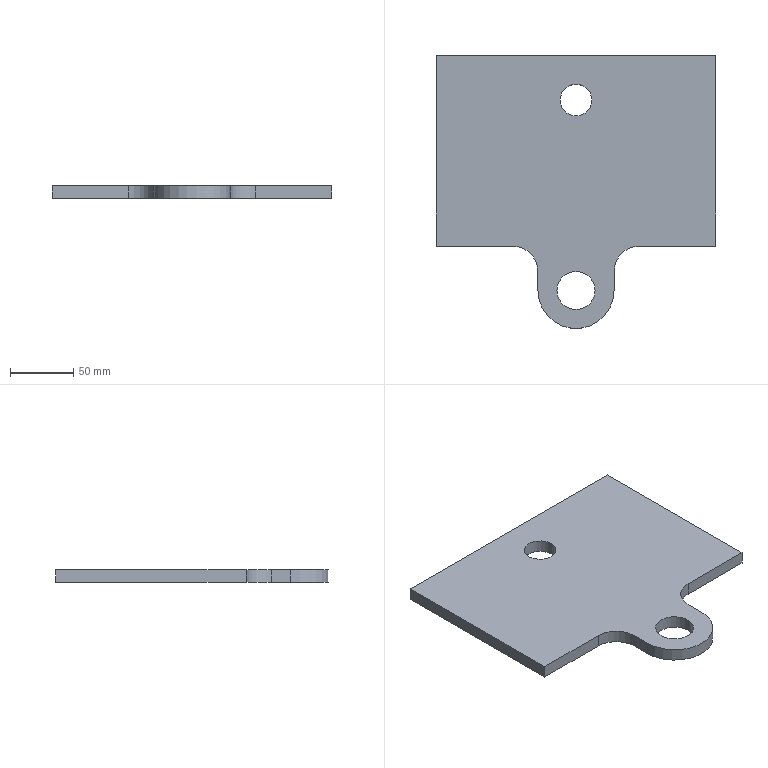Part | SolidWorks | features Extrusion 1, Fillet 1 | 1 solid | 16 faces | box 220 x 215 x 10 mm | volume 354877 mm3 | plane 9 | cylinder 7 | commonest cylinder face diameters 25 x2 30 x2 40 x2 60 x1
STEP:
#1=CARTESIAN_POINT('',(-12.5,40.,5.));
#2=VERTEX_POINT('',#1);
#3=CARTESIAN_POINT('',(12.5,40.,5.));
#4=VERTEX_POINT('',#3);
#5=CARTESIAN_POINT('',(0.,40.,5.));
#6=DIRECTION('',(0.,0.,1.));
#7=DIRECTION('',(1.,0.,0.));
#8=AXIS2_PLACEMENT_3D('',#5,#6,#7);
#9=CIRCLE('',#8,12.5);
#10=EDGE_CURVE('',#2,#4,#9,.T.);
#11=ORIENTED_EDGE('',*,*,#10,.T.);
#12=CARTESIAN_POINT('',(12.5,40.,-5.));
#13=VERTEX_POINT('',#12);
#14=CARTESIAN_POINT('',(12.5,40.,5.));
#15=DIRECTION('',(0.,0.,-1.));
#16=VECTOR('',#15,1000.);
#17=LINE('',#14,#16);
#18=EDGE_CURVE('',#4,#13,#17,.T.);
#19=ORIENTED_EDGE('',*,*,#18,.T.);
#20=CARTESIAN_POINT('',(-12.5,40.,-5.));
#21=VERTEX_POINT('',#20);
#22=CARTESIAN_POINT('',(0.,40.,-5.));
#23=DIRECTION('',(0.,0.,1.));
#24=DIRECTION('',(1.,0.,0.));
#25=AXIS2_PLACEMENT_3D('',#22,#23,#24);
#26=CIRCLE('',#25,12.5);
#27=EDGE_CURVE('',#21,#13,#26,.T.);
#28=ORIENTED_EDGE('',*,*,#27,.F.);
#29=CARTESIAN_POINT('',(-12.5,40.,5.));
#30=DIRECTION('',(0.,0.,-1.));
#31=VECTOR('',#30,1000.);
#32=LINE('',#29,#31);
#33=EDGE_CURVE('',#2,#21,#32,.T.);
#34=ORIENTED_EDGE('',*,*,#33,.F.);
#35=EDGE_LOOP('',(#11,#19,#28,#34));
#36=FACE_OUTER_BOUND('',#35,.T.);
#37=CARTESIAN_POINT('',(0.,40.,5.));
#38=DIRECTION('',(0.,0.,-1.));
#39=DIRECTION('',(-1.,0.,0.));
#40=AXIS2_PLACEMENT_3D('',#37,#38,#39);
#41=CYLINDRICAL_SURFACE('',#40,12.5);
#42=ADVANCED_FACE('',(#36),#41,.F.);
#43=CARTESIAN_POINT('',(-15.,-110.,5.));
#44=VERTEX_POINT('',#43);
#45=CARTESIAN_POINT('',(15.,-110.,5.));
#46=VERTEX_POINT('',#45);
#47=CARTESIAN_POINT('',(0.,-110.,5.));
#48=DIRECTION('',(0.,0.,1.));
#49=DIRECTION('',(1.,0.,0.));
#50=AXIS2_PLACEMENT_3D('',#47,#48,#49);
#51=CIRCLE('',#50,15.);
#52=EDGE_CURVE('',#44,#46,#51,.T.);
#53=ORIENTED_EDGE('',*,*,#52,.T.);
#54=CARTESIAN_POINT('',(15.,-110.,-5.));
#55=VERTEX_POINT('',#54);
#56=CARTESIAN_POINT('',(15.,-110.,5.));
#57=DIRECTION('',(0.,0.,-1.));
#58=VECTOR('',#57,1000.);
#59=LINE('',#56,#58);
#60=EDGE_CURVE('',#46,#55,#59,.T.);
#61=ORIENTED_EDGE('',*,*,#60,.T.);
#62=CARTESIAN_POINT('',(-15.,-110.,-5.));
#63=VERTEX_POINT('',#62);
#64=CARTESIAN_POINT('',(0.,-110.,-5.));
#65=DIRECTION('',(0.,0.,1.));
#66=DIRECTION('',(1.,0.,0.));
#67=AXIS2_PLACEMENT_3D('',#64,#65,#66);
#68=CIRCLE('',#67,15.);
#69=EDGE_CURVE('',#63,#55,#68,.T.);
#70=ORIENTED_EDGE('',*,*,#69,.F.);
#71=CARTESIAN_POINT('',(-15.,-110.,5.));
#72=DIRECTION('',(0.,0.,-1.));
#73=VECTOR('',#72,1000.);
#74=LINE('',#71,#73);
#75=EDGE_CURVE('',#44,#63,#74,.T.);
#76=ORIENTED_EDGE('',*,*,#75,.F.);
#77=EDGE_LOOP('',(#53,#61,#70,#76));
#78=FACE_OUTER_BOUND('',#77,.T.);
#79=CARTESIAN_POINT('',(0.,-110.,5.));
#80=DIRECTION('',(0.,0.,-1.));
#81=DIRECTION('',(-1.,0.,0.));
#82=AXIS2_PLACEMENT_3D('',#79,#80,#81);
#83=CYLINDRICAL_SURFACE('',#82,15.);
#84=ADVANCED_FACE('',(#78),#83,.F.);
#85=CARTESIAN_POINT('',(-30.,-95.,5.));
#86=VERTEX_POINT('',#85);
#87=CARTESIAN_POINT('',(-30.,-110.,5.));
#88=VERTEX_POINT('',#87);
#89=CARTESIAN_POINT('',(-30.,0.,5.));
#90=DIRECTION('',(0.,-1.,0.));
#91=VECTOR('',#90,1000.);
#92=LINE('',#89,#91);
#93=EDGE_CURVE('',#86,#88,#92,.T.);
#94=ORIENTED_EDGE('',*,*,#93,.F.);
#95=CARTESIAN_POINT('',(-30.,-95.,-5.));
#96=VERTEX_POINT('',#95);
#97=CARTESIAN_POINT('',(-30.,-95.,5.));
#98=DIRECTION('',(0.,0.,-1.));
#99=VECTOR('',#98,1000.);
#100=LINE('',#97,#99);
#101=EDGE_CURVE('',#86,#96,#100,.T.);
#102=ORIENTED_EDGE('',*,*,#101,.T.);
#103=CARTESIAN_POINT('',(-30.,-110.,-5.));
#104=VERTEX_POINT('',#103);
#105=CARTESIAN_POINT('',(-30.,0.,-5.));
#106=DIRECTION('',(0.,-1.,0.));
#107=VECTOR('',#106,1000.);
#108=LINE('',#105,#107);
#109=EDGE_CURVE('',#96,#104,#108,.T.);
#110=ORIENTED_EDGE('',*,*,#109,.T.);
#111=CARTESIAN_POINT('',(-30.,-110.,5.));
#112=DIRECTION('',(0.,0.,-1.));
#113=VECTOR('',#112,1000.);
#114=LINE('',#111,#113);
#115=EDGE_CURVE('',#88,#104,#114,.T.);
#116=ORIENTED_EDGE('',*,*,#115,.F.);
#117=EDGE_LOOP('',(#94,#102,#110,#116));
#118=FACE_OUTER_BOUND('',#117,.T.);
#119=CARTESIAN_POINT('',(-30.,0.,5.));
#120=DIRECTION('',(1.,0.,0.));
#121=DIRECTION('',(0.,0.,-1.));
#122=AXIS2_PLACEMENT_3D('',#119,#120,#121);
#123=PLANE('',#122);
#124=ADVANCED_FACE('',(#118),#123,.F.);
#125=CARTESIAN_POINT('',(30.,-110.,-5.));
#126=VERTEX_POINT('',#125);
#127=CARTESIAN_POINT('',(0.,-110.,-5.));
#128=DIRECTION('',(0.,0.,1.));
#129=DIRECTION('',(1.,0.,0.));
#130=AXIS2_PLACEMENT_3D('',#127,#128,#129);
#131=CIRCLE('',#130,30.);
#132=EDGE_CURVE('',#104,#126,#131,.T.);
#133=ORIENTED_EDGE('',*,*,#132,.T.);
#134=CARTESIAN_POINT('',(30.,-110.,5.));
#135=VERTEX_POINT('',#134);
#136=CARTESIAN_POINT('',(30.,-110.,5.));
#137=DIRECTION('',(0.,0.,-1.));
#138=VECTOR('',#137,1000.);
#139=LINE('',#136,#138);
#140=EDGE_CURVE('',#135,#126,#139,.T.);
#141=ORIENTED_EDGE('',*,*,#140,.F.);
#142=CARTESIAN_POINT('',(0.,-110.,5.));
#143=DIRECTION('',(0.,0.,1.));
#144=DIRECTION('',(1.,0.,0.));
#145=AXIS2_PLACEMENT_3D('',#142,#143,#144);
#146=CIRCLE('',#145,30.);
#147=EDGE_CURVE('',#88,#135,#146,.T.);
#148=ORIENTED_EDGE('',*,*,#147,.F.);
#149=ORIENTED_EDGE('',*,*,#115,.T.);
#150=EDGE_LOOP('',(#133,#141,#148,#149));
#151=FACE_OUTER_BOUND('',#150,.T.);
#152=CARTESIAN_POINT('',(0.,-110.,5.));
#153=DIRECTION('',(0.,0.,-1.));
#154=DIRECTION('',(-1.,0.,0.));
#155=AXIS2_PLACEMENT_3D('',#152,#153,#154);
#156=CYLINDRICAL_SURFACE('',#155,30.);
#157=ADVANCED_FACE('',(#151),#156,.T.);
#158=CARTESIAN_POINT('',(30.,-95.,-5.));
#159=VERTEX_POINT('',#158);
#160=CARTESIAN_POINT('',(30.,0.,-5.));
#161=DIRECTION('',(0.,-1.,0.));
#162=VECTOR('',#161,1000.);
#163=LINE('',#160,#162);
#164=EDGE_CURVE('',#159,#126,#163,.T.);
#165=ORIENTED_EDGE('',*,*,#164,.F.);
#166=CARTESIAN_POINT('',(30.,-95.,5.));
#167=VERTEX_POINT('',#166);
#168=CARTESIAN_POINT('',(30.,-95.,5.));
#169=DIRECTION('',(0.,0.,1.));
#170=VECTOR('',#169,1000.);
#171=LINE('',#168,#170);
#172=EDGE_CURVE('',#159,#167,#171,.T.);
#173=ORIENTED_EDGE('',*,*,#172,.T.);
#174=CARTESIAN_POINT('',(30.,0.,5.));
#175=DIRECTION('',(0.,-1.,0.));
#176=VECTOR('',#175,1000.);
#177=LINE('',#174,#176);
#178=EDGE_CURVE('',#167,#135,#177,.T.);
#179=ORIENTED_EDGE('',*,*,#178,.T.);
#180=ORIENTED_EDGE('',*,*,#140,.T.);
#181=EDGE_LOOP('',(#165,#173,#179,#180));
#182=FACE_OUTER_BOUND('',#181,.T.);
#183=CARTESIAN_POINT('',(30.,0.,5.));
#184=DIRECTION('',(1.,0.,0.));
#185=DIRECTION('',(0.,0.,-1.));
#186=AXIS2_PLACEMENT_3D('',#183,#184,#185);
#187=PLANE('',#186);
#188=ADVANCED_FACE('',(#182),#187,.T.);
#189=CARTESIAN_POINT('',(110.,-75.,5.));
#190=VERTEX_POINT('',#189);
#191=CARTESIAN_POINT('',(50.,-75.,5.));
#192=VERTEX_POINT('',#191);
#193=CARTESIAN_POINT('',(0.,-75.,5.));
#194=DIRECTION('',(-1.,0.,0.));
#195=VECTOR('',#194,1000.);
#196=LINE('',#193,#195);
#197=EDGE_CURVE('',#190,#192,#196,.T.);
#198=ORIENTED_EDGE('',*,*,#197,.T.);
#199=CARTESIAN_POINT('',(50.,-75.,-5.));
#200=VERTEX_POINT('',#199);
#201=CARTESIAN_POINT('',(50.,-75.,-5.));
#202=DIRECTION('',(0.,0.,-1.));
#203=VECTOR('',#202,1000.);
#204=LINE('',#201,#203);
#205=EDGE_CURVE('',#192,#200,#204,.T.);
#206=ORIENTED_EDGE('',*,*,#205,.T.);
#207=CARTESIAN_POINT('',(110.,-75.,-5.));
#208=VERTEX_POINT('',#207);
#209=CARTESIAN_POINT('',(0.,-75.,-5.));
#210=DIRECTION('',(-1.,0.,0.));
#211=VECTOR('',#210,1000.);
#212=LINE('',#209,#211);
#213=EDGE_CURVE('',#208,#200,#212,.T.);
#214=ORIENTED_EDGE('',*,*,#213,.F.);
#215=CARTESIAN_POINT('',(110.,-75.,5.));
#216=DIRECTION('',(0.,0.,-1.));
#217=VECTOR('',#216,1000.);
#218=LINE('',#215,#217);
#219=EDGE_CURVE('',#190,#208,#218,.T.);
#220=ORIENTED_EDGE('',*,*,#219,.F.);
#221=EDGE_LOOP('',(#198,#206,#214,#220));
#222=FACE_OUTER_BOUND('',#221,.T.);
#223=CARTESIAN_POINT('',(0.,-75.,5.));
#224=DIRECTION('',(0.,-1.,0.));
#225=DIRECTION('',(1.,0.,0.));
#226=AXIS2_PLACEMENT_3D('',#223,#224,#225);
#227=PLANE('',#226);
#228=ADVANCED_FACE('',(#222),#227,.T.);
#229=CARTESIAN_POINT('',(110.,75.,-5.));
#230=VERTEX_POINT('',#229);
#231=CARTESIAN_POINT('',(110.,0.,-5.));
#232=DIRECTION('',(0.,1.,0.));
#233=VECTOR('',#232,1000.);
#234=LINE('',#231,#233);
#235=EDGE_CURVE('',#208,#230,#234,.T.);
#236=ORIENTED_EDGE('',*,*,#235,.T.);
#237=CARTESIAN_POINT('',(110.,75.,5.));
#238=VERTEX_POINT('',#237);
#239=CARTESIAN_POINT('',(110.,75.,5.));
#240=DIRECTION('',(0.,0.,-1.));
#241=VECTOR('',#240,1000.);
#242=LINE('',#239,#241);
#243=EDGE_CURVE('',#238,#230,#242,.T.);
#244=ORIENTED_EDGE('',*,*,#243,.F.);
#245=CARTESIAN_POINT('',(110.,0.,5.));
#246=DIRECTION('',(0.,1.,0.));
#247=VECTOR('',#246,1000.);
#248=LINE('',#245,#247);
#249=EDGE_CURVE('',#190,#238,#248,.T.);
#250=ORIENTED_EDGE('',*,*,#249,.F.);
#251=ORIENTED_EDGE('',*,*,#219,.T.);
#252=EDGE_LOOP('',(#236,#244,#250,#251));
#253=FACE_OUTER_BOUND('',#252,.T.);
#254=CARTESIAN_POINT('',(110.,0.,5.));
#255=DIRECTION('',(-1.,0.,0.));
#256=DIRECTION('',(0.,-1.,0.));
#257=AXIS2_PLACEMENT_3D('',#254,#255,#256);
#258=PLANE('',#257);
#259=ADVANCED_FACE('',(#253),#258,.F.);
#260=CARTESIAN_POINT('',(-110.,75.,-5.));
#261=VERTEX_POINT('',#260);
#262=CARTESIAN_POINT('',(0.,75.,-5.));
#263=DIRECTION('',(-1.,0.,0.));
#264=VECTOR('',#263,1000.);
#265=LINE('',#262,#264);
#266=EDGE_CURVE('',#230,#261,#265,.T.);
#267=ORIENTED_EDGE('',*,*,#266,.T.);
#268=CARTESIAN_POINT('',(-110.,75.,5.));
#269=VERTEX_POINT('',#268);
#270=CARTESIAN_POINT('',(-110.,75.,5.));
#271=DIRECTION('',(0.,0.,-1.));
#272=VECTOR('',#271,1000.);
#273=LINE('',#270,#272);
#274=EDGE_CURVE('',#269,#261,#273,.T.);
#275=ORIENTED_EDGE('',*,*,#274,.F.);
#276=CARTESIAN_POINT('',(0.,75.,5.));
#277=DIRECTION('',(-1.,0.,0.));
#278=VECTOR('',#277,1000.);
#279=LINE('',#276,#278);
#280=EDGE_CURVE('',#238,#269,#279,.T.);
#281=ORIENTED_EDGE('',*,*,#280,.F.);
#282=ORIENTED_EDGE('',*,*,#243,.T.);
#283=EDGE_LOOP('',(#267,#275,#281,#282));
#284=FACE_OUTER_BOUND('',#283,.T.);
#285=CARTESIAN_POINT('',(0.,75.,5.));
#286=DIRECTION('',(0.,-1.,0.));
#287=DIRECTION('',(0.,0.,-1.));
#288=AXIS2_PLACEMENT_3D('',#285,#286,#287);
#289=PLANE('',#288);
#290=ADVANCED_FACE('',(#284),#289,.F.);
#291=CARTESIAN_POINT('',(-110.,-75.,-5.));
#292=VERTEX_POINT('',#291);
#293=CARTESIAN_POINT('',(-110.,0.,-5.));
#294=DIRECTION('',(0.,1.,0.));
#295=VECTOR('',#294,1000.);
#296=LINE('',#293,#295);
#297=EDGE_CURVE('',#292,#261,#296,.T.);
#298=ORIENTED_EDGE('',*,*,#297,.F.);
#299=CARTESIAN_POINT('',(-110.,-75.,5.));
#300=VERTEX_POINT('',#299);
#301=CARTESIAN_POINT('',(-110.,-75.,5.));
#302=DIRECTION('',(0.,0.,-1.));
#303=VECTOR('',#302,1000.);
#304=LINE('',#301,#303);
#305=EDGE_CURVE('',#300,#292,#304,.T.);
#306=ORIENTED_EDGE('',*,*,#305,.F.);
#307=CARTESIAN_POINT('',(-110.,0.,5.));
#308=DIRECTION('',(0.,1.,0.));
#309=VECTOR('',#308,1000.);
#310=LINE('',#307,#309);
#311=EDGE_CURVE('',#300,#269,#310,.T.);
#312=ORIENTED_EDGE('',*,*,#311,.T.);
#313=ORIENTED_EDGE('',*,*,#274,.T.);
#314=EDGE_LOOP('',(#298,#306,#312,#313));
#315=FACE_OUTER_BOUND('',#314,.T.);
#316=CARTESIAN_POINT('',(-110.,0.,5.));
#317=DIRECTION('',(-1.,0.,0.));
#318=DIRECTION('',(0.,0.,1.));
#319=AXIS2_PLACEMENT_3D('',#316,#317,#318);
#320=PLANE('',#319);
#321=ADVANCED_FACE('',(#315),#320,.T.);
#322=CARTESIAN_POINT('',(-50.,-75.,-5.));
#323=VERTEX_POINT('',#322);
#324=CARTESIAN_POINT('',(0.,-75.,-5.));
#325=DIRECTION('',(-1.,0.,0.));
#326=VECTOR('',#325,1000.);
#327=LINE('',#324,#326);
#328=EDGE_CURVE('',#323,#292,#327,.T.);
#329=ORIENTED_EDGE('',*,*,#328,.F.);
#330=CARTESIAN_POINT('',(-50.,-75.,5.));
#331=VERTEX_POINT('',#330);
#332=CARTESIAN_POINT('',(-50.,-75.,5.));
#333=DIRECTION('',(0.,0.,1.));
#334=VECTOR('',#333,1000.);
#335=LINE('',#332,#334);
#336=EDGE_CURVE('',#323,#331,#335,.T.);
#337=ORIENTED_EDGE('',*,*,#336,.T.);
#338=CARTESIAN_POINT('',(0.,-75.,5.));
#339=DIRECTION('',(-1.,0.,0.));
#340=VECTOR('',#339,1000.);
#341=LINE('',#338,#340);
#342=EDGE_CURVE('',#331,#300,#341,.T.);
#343=ORIENTED_EDGE('',*,*,#342,.T.);
#344=ORIENTED_EDGE('',*,*,#305,.T.);
#345=EDGE_LOOP('',(#329,#337,#343,#344));
#346=FACE_OUTER_BOUND('',#345,.T.);
#347=CARTESIAN_POINT('',(0.,-75.,5.));
#348=DIRECTION('',(0.,-1.,0.));
#349=DIRECTION('',(1.,0.,0.));
#350=AXIS2_PLACEMENT_3D('',#347,#348,#349);
#351=PLANE('',#350);
#352=ADVANCED_FACE('',(#346),#351,.T.);
#353=ORIENTED_EDGE('',*,*,#60,.F.);
#354=CARTESIAN_POINT('',(0.,-110.,5.));
#355=DIRECTION('',(0.,0.,1.));
#356=DIRECTION('',(1.,0.,0.));
#357=AXIS2_PLACEMENT_3D('',#354,#355,#356);
#358=CIRCLE('',#357,15.);
#359=EDGE_CURVE('',#46,#44,#358,.T.);
#360=ORIENTED_EDGE('',*,*,#359,.T.);
#361=ORIENTED_EDGE('',*,*,#75,.T.);
#362=CARTESIAN_POINT('',(0.,-110.,-5.));
#363=DIRECTION('',(0.,0.,1.));
#364=DIRECTION('',(1.,0.,0.));
#365=AXIS2_PLACEMENT_3D('',#362,#363,#364);
#366=CIRCLE('',#365,15.);
#367=EDGE_CURVE('',#55,#63,#366,.T.);
#368=ORIENTED_EDGE('',*,*,#367,.F.);
#369=EDGE_LOOP('',(#353,#360,#361,#368));
#370=FACE_OUTER_BOUND('',#369,.T.);
#371=CARTESIAN_POINT('',(0.,-110.,5.));
#372=DIRECTION('',(0.,0.,-1.));
#373=DIRECTION('',(-1.,0.,0.));
#374=AXIS2_PLACEMENT_3D('',#371,#372,#373);
#375=CYLINDRICAL_SURFACE('',#374,15.);
#376=ADVANCED_FACE('',(#370),#375,.F.);
#377=ORIENTED_EDGE('',*,*,#18,.F.);
#378=CARTESIAN_POINT('',(0.,40.,5.));
#379=DIRECTION('',(0.,0.,1.));
#380=DIRECTION('',(1.,0.,0.));
#381=AXIS2_PLACEMENT_3D('',#378,#379,#380);
#382=CIRCLE('',#381,12.5);
#383=EDGE_CURVE('',#4,#2,#382,.T.);
#384=ORIENTED_EDGE('',*,*,#383,.T.);
#385=ORIENTED_EDGE('',*,*,#33,.T.);
#386=CARTESIAN_POINT('',(0.,40.,-5.));
#387=DIRECTION('',(0.,0.,1.));
#388=DIRECTION('',(1.,0.,0.));
#389=AXIS2_PLACEMENT_3D('',#386,#387,#388);
#390=CIRCLE('',#389,12.5);
#391=EDGE_CURVE('',#13,#21,#390,.T.);
#392=ORIENTED_EDGE('',*,*,#391,.F.);
#393=EDGE_LOOP('',(#377,#384,#385,#392));
#394=FACE_OUTER_BOUND('',#393,.T.);
#395=CARTESIAN_POINT('',(0.,40.,5.));
#396=DIRECTION('',(0.,0.,-1.));
#397=DIRECTION('',(-1.,0.,0.));
#398=AXIS2_PLACEMENT_3D('',#395,#396,#397);
#399=CYLINDRICAL_SURFACE('',#398,12.5);
#400=ADVANCED_FACE('',(#394),#399,.F.);
#401=ORIENTED_EDGE('',*,*,#52,.F.);
#402=ORIENTED_EDGE('',*,*,#359,.F.);
#403=EDGE_LOOP('',(#401,#402));
#404=FACE_BOUND('',#403,.T.);
#405=ORIENTED_EDGE('',*,*,#342,.F.);
#406=CARTESIAN_POINT('',(-50.,-95.,5.));
#407=DIRECTION('',(0.,0.,-1.));
#408=DIRECTION('',(1.,0.,0.));
#409=AXIS2_PLACEMENT_3D('',#406,#407,#408);
#410=CIRCLE('',#409,20.);
#411=EDGE_CURVE('',#331,#86,#410,.T.);
#412=ORIENTED_EDGE('',*,*,#411,.T.);
#413=ORIENTED_EDGE('',*,*,#93,.T.);
#414=ORIENTED_EDGE('',*,*,#147,.T.);
#415=ORIENTED_EDGE('',*,*,#178,.F.);
#416=CARTESIAN_POINT('',(50.,-95.,5.));
#417=DIRECTION('',(0.,0.,-1.));
#418=DIRECTION('',(1.,0.,0.));
#419=AXIS2_PLACEMENT_3D('',#416,#417,#418);
#420=CIRCLE('',#419,20.);
#421=EDGE_CURVE('',#167,#192,#420,.T.);
#422=ORIENTED_EDGE('',*,*,#421,.T.);
#423=ORIENTED_EDGE('',*,*,#197,.F.);
#424=ORIENTED_EDGE('',*,*,#249,.T.);
#425=ORIENTED_EDGE('',*,*,#280,.T.);
#426=ORIENTED_EDGE('',*,*,#311,.F.);
#427=EDGE_LOOP('',(#405,#412,#413,#414,#415,#422,#423,#424,#425,#426));
#428=FACE_OUTER_BOUND('',#427,.T.);
#429=ORIENTED_EDGE('',*,*,#10,.F.);
#430=ORIENTED_EDGE('',*,*,#383,.F.);
#431=EDGE_LOOP('',(#429,#430));
#432=FACE_BOUND('',#431,.T.);
#433=CARTESIAN_POINT('',(0.,0.,5.));
#434=DIRECTION('',(0.,0.,1.));
#435=DIRECTION('',(1.,0.,0.));
#436=AXIS2_PLACEMENT_3D('',#433,#434,#435);
#437=PLANE('',#436);
#438=ADVANCED_FACE('',(#404,#428,#432),#437,.T.);
#439=ORIENTED_EDGE('',*,*,#69,.T.);
#440=ORIENTED_EDGE('',*,*,#367,.T.);
#441=EDGE_LOOP('',(#439,#440));
#442=FACE_BOUND('',#441,.T.);
#443=ORIENTED_EDGE('',*,*,#109,.F.);
#444=CARTESIAN_POINT('',(-50.,-95.,-5.));
#445=DIRECTION('',(0.,0.,1.));
#446=DIRECTION('',(1.,0.,0.));
#447=AXIS2_PLACEMENT_3D('',#444,#445,#446);
#448=CIRCLE('',#447,20.);
#449=EDGE_CURVE('',#96,#323,#448,.T.);
#450=ORIENTED_EDGE('',*,*,#449,.T.);
#451=ORIENTED_EDGE('',*,*,#328,.T.);
#452=ORIENTED_EDGE('',*,*,#297,.T.);
#453=ORIENTED_EDGE('',*,*,#266,.F.);
#454=ORIENTED_EDGE('',*,*,#235,.F.);
#455=ORIENTED_EDGE('',*,*,#213,.T.);
#456=CARTESIAN_POINT('',(50.,-95.,-5.));
#457=DIRECTION('',(0.,0.,1.));
#458=DIRECTION('',(1.,0.,0.));
#459=AXIS2_PLACEMENT_3D('',#456,#457,#458);
#460=CIRCLE('',#459,20.);
#461=EDGE_CURVE('',#200,#159,#460,.T.);
#462=ORIENTED_EDGE('',*,*,#461,.T.);
#463=ORIENTED_EDGE('',*,*,#164,.T.);
#464=ORIENTED_EDGE('',*,*,#132,.F.);
#465=EDGE_LOOP('',(#443,#450,#451,#452,#453,#454,#455,#462,#463,#464));
#466=FACE_OUTER_BOUND('',#465,.T.);
#467=ORIENTED_EDGE('',*,*,#27,.T.);
#468=ORIENTED_EDGE('',*,*,#391,.T.);
#469=EDGE_LOOP('',(#467,#468));
#470=FACE_BOUND('',#469,.T.);
#471=CARTESIAN_POINT('',(0.,0.,-5.));
#472=DIRECTION('',(0.,0.,1.));
#473=DIRECTION('',(1.,0.,0.));
#474=AXIS2_PLACEMENT_3D('',#471,#472,#473);
#475=PLANE('',#474);
#476=ADVANCED_FACE('',(#442,#466,#470),#475,.F.);
#477=ORIENTED_EDGE('',*,*,#411,.F.);
#478=ORIENTED_EDGE('',*,*,#336,.F.);
#479=ORIENTED_EDGE('',*,*,#449,.F.);
#480=ORIENTED_EDGE('',*,*,#101,.F.);
#481=EDGE_LOOP('',(#477,#478,#479,#480));
#482=FACE_OUTER_BOUND('',#481,.T.);
#483=CARTESIAN_POINT('',(-50.,-95.,5.));
#484=DIRECTION('',(0.,0.,-1.));
#485=DIRECTION('',(-1.,0.,0.));
#486=AXIS2_PLACEMENT_3D('',#483,#484,#485);
#487=CYLINDRICAL_SURFACE('',#486,20.);
#488=ADVANCED_FACE('',(#482),#487,.F.);
#489=ORIENTED_EDGE('',*,*,#421,.F.);
#490=ORIENTED_EDGE('',*,*,#172,.F.);
#491=ORIENTED_EDGE('',*,*,#461,.F.);
#492=ORIENTED_EDGE('',*,*,#205,.F.);
#493=EDGE_LOOP('',(#489,#490,#491,#492));
#494=FACE_OUTER_BOUND('',#493,.T.);
#495=CARTESIAN_POINT('',(50.,-95.,5.));
#496=DIRECTION('',(0.,0.,1.));
#497=DIRECTION('',(1.,0.,0.));
#498=AXIS2_PLACEMENT_3D('',#495,#496,#497);
#499=CYLINDRICAL_SURFACE('',#498,20.);
#500=ADVANCED_FACE('',(#494),#499,.F.);
#501=CLOSED_SHELL('',(#42,#84,#124,#157,#188,#228,#259,#290,#321,#352,#376,#400,#438,#476,#488,#500));
#502=MANIFOLD_SOLID_BREP('',#501);
#503=CARTESIAN_POINT('',(0.,0.,0.));
#504=DIRECTION('',(0.,0.,1.));
#505=DIRECTION('',(1.,0.,0.));
#506=AXIS2_PLACEMENT_3D('',#503,#504,#505);
#507=(LENGTH_UNIT()NAMED_UNIT(*)SI_UNIT(.MILLI.,.METRE.));
#508=UNCERTAINTY_MEASURE_WITH_UNIT(LENGTH_MEASURE(0.00001),#507,'','');
#509=(NAMED_UNIT(*)PLANE_ANGLE_UNIT()SI_UNIT($,.RADIAN.));
#510=(NAMED_UNIT(*)SI_UNIT($,.STERADIAN.)SOLID_ANGLE_UNIT());
#511=(GEOMETRIC_REPRESENTATION_CONTEXT(3)GLOBAL_UNCERTAINTY_ASSIGNED_CONTEXT((#508))GLOBAL_UNIT_ASSIGNED_CONTEXT((#507,#509,#510))REPRESENTATION_CONTEXT('',''));
#512=ADVANCED_BREP_SHAPE_REPRESENTATION('',(#502,#506),#511);